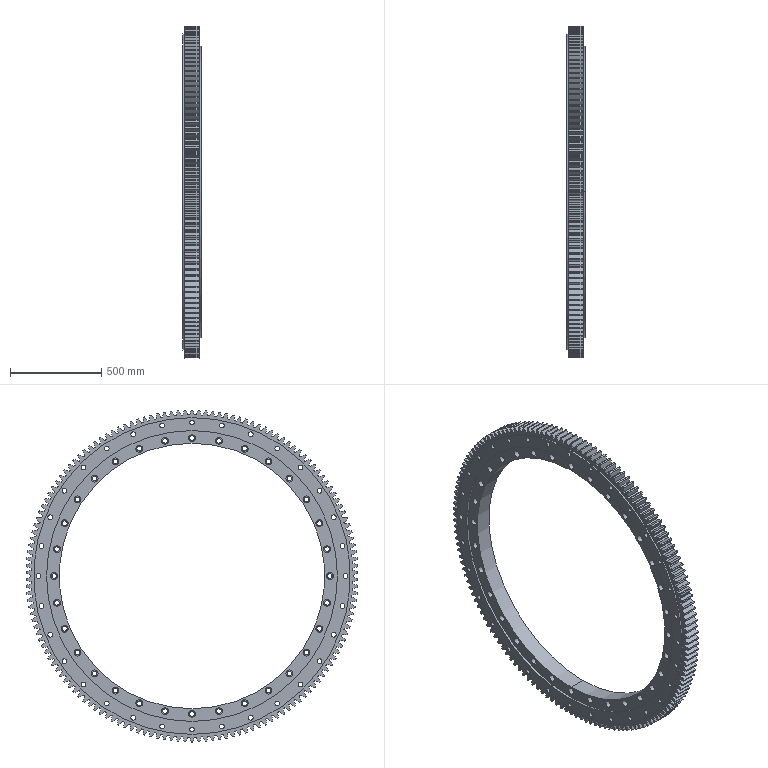Part | SolidWorks | features ICE 4, SketchHole 4, CirPattern 1, Stock 1 | 1 solid | 938 faces | box 102 x 1824 x 1824 mm | volume 72400415 mm3 | cylinder 869 | plane 69 | commonest cylinder face diameters 720 x304 1824 x151 1770 x150 26 x128 38 x128 1458 x2